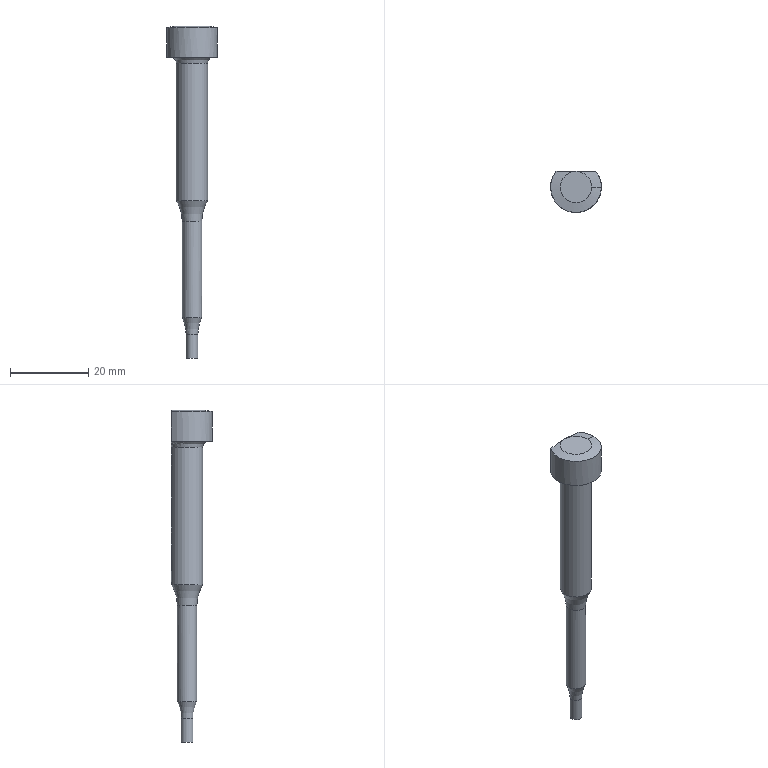Part | NX | features MI_APTWA_0168 2 | 1 solid | 470 faces | box 13 x 10.5 x 85 mm | volume 3484 mm3 | plane 286 | cylinder 178 | spline 3 | torus 2 | cone 1 | commonest cylinder face diameters 7.8 x37 8 x18 0.509 x6 0.608 x6 0.61 x6 0.617 x6